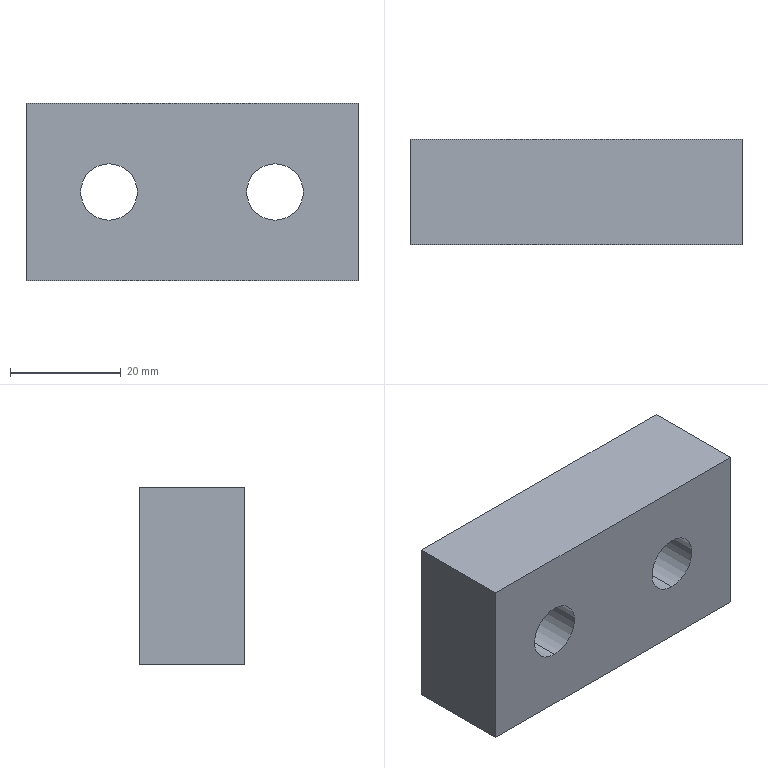Part | SolidWorks | features FlatPattern 1, HoleWzd 1, SMBaseFlange 1, SheetMetal 1 | 1 solid | 10 faces | box 60 x 19 x 32 mm | volume 33375 mm3 | plane 6 | cylinder 4 | commonest cylinder face diameters 10.2 x4
STEP:
#1=CARTESIAN_POINT('',(-15.,-19.,-5.1));
#2=VERTEX_POINT('',#1);
#3=CARTESIAN_POINT('',(-15.,-19.,5.1));
#4=VERTEX_POINT('',#3);
#5=CARTESIAN_POINT('',(-15.,-19.,0.));
#6=DIRECTION('',(0.,1.,0.));
#7=DIRECTION('',(0.,0.,1.));
#8=AXIS2_PLACEMENT_3D('',#5,#6,#7);
#9=CIRCLE('',#8,5.1);
#10=EDGE_CURVE('',#2,#4,#9,.T.);
#11=ORIENTED_EDGE('',*,*,#10,.F.);
#12=CARTESIAN_POINT('',(-15.,0.,-5.1));
#13=VERTEX_POINT('',#12);
#14=CARTESIAN_POINT('',(-15.,0.,-5.1));
#15=DIRECTION('',(0.,1.,0.));
#16=VECTOR('',#15,1000.);
#17=LINE('',#14,#16);
#18=EDGE_CURVE('',#2,#13,#17,.T.);
#19=ORIENTED_EDGE('',*,*,#18,.T.);
#20=CARTESIAN_POINT('',(-15.,0.,5.1));
#21=VERTEX_POINT('',#20);
#22=CARTESIAN_POINT('',(-15.,0.,0.));
#23=DIRECTION('',(0.,1.,0.));
#24=DIRECTION('',(0.,0.,1.));
#25=AXIS2_PLACEMENT_3D('',#22,#23,#24);
#26=CIRCLE('',#25,5.1);
#27=EDGE_CURVE('',#13,#21,#26,.T.);
#28=ORIENTED_EDGE('',*,*,#27,.T.);
#29=CARTESIAN_POINT('',(-15.,0.,5.1));
#30=DIRECTION('',(0.,1.,0.));
#31=VECTOR('',#30,1000.);
#32=LINE('',#29,#31);
#33=EDGE_CURVE('',#4,#21,#32,.T.);
#34=ORIENTED_EDGE('',*,*,#33,.F.);
#35=EDGE_LOOP('',(#11,#19,#28,#34));
#36=FACE_OUTER_BOUND('',#35,.T.);
#37=CARTESIAN_POINT('',(-15.,0.,0.));
#38=DIRECTION('',(0.,1.,0.));
#39=DIRECTION('',(0.,0.,1.));
#40=AXIS2_PLACEMENT_3D('',#37,#38,#39);
#41=CYLINDRICAL_SURFACE('',#40,5.1);
#42=ADVANCED_FACE('',(#36),#41,.F.);
#43=CARTESIAN_POINT('',(15.,-19.,-5.1));
#44=VERTEX_POINT('',#43);
#45=CARTESIAN_POINT('',(15.,-19.,5.1));
#46=VERTEX_POINT('',#45);
#47=CARTESIAN_POINT('',(15.,-19.,0.));
#48=DIRECTION('',(0.,1.,0.));
#49=DIRECTION('',(0.,0.,1.));
#50=AXIS2_PLACEMENT_3D('',#47,#48,#49);
#51=CIRCLE('',#50,5.1);
#52=EDGE_CURVE('',#44,#46,#51,.T.);
#53=ORIENTED_EDGE('',*,*,#52,.F.);
#54=CARTESIAN_POINT('',(15.,0.,-5.1));
#55=VERTEX_POINT('',#54);
#56=CARTESIAN_POINT('',(15.,0.,-5.1));
#57=DIRECTION('',(0.,1.,0.));
#58=VECTOR('',#57,1000.);
#59=LINE('',#56,#58);
#60=EDGE_CURVE('',#44,#55,#59,.T.);
#61=ORIENTED_EDGE('',*,*,#60,.T.);
#62=CARTESIAN_POINT('',(15.,0.,5.1));
#63=VERTEX_POINT('',#62);
#64=CARTESIAN_POINT('',(15.,0.,0.));
#65=DIRECTION('',(0.,1.,0.));
#66=DIRECTION('',(0.,0.,1.));
#67=AXIS2_PLACEMENT_3D('',#64,#65,#66);
#68=CIRCLE('',#67,5.1);
#69=EDGE_CURVE('',#55,#63,#68,.T.);
#70=ORIENTED_EDGE('',*,*,#69,.T.);
#71=CARTESIAN_POINT('',(15.,0.,5.1));
#72=DIRECTION('',(0.,1.,0.));
#73=VECTOR('',#72,1000.);
#74=LINE('',#71,#73);
#75=EDGE_CURVE('',#46,#63,#74,.T.);
#76=ORIENTED_EDGE('',*,*,#75,.F.);
#77=EDGE_LOOP('',(#53,#61,#70,#76));
#78=FACE_OUTER_BOUND('',#77,.T.);
#79=CARTESIAN_POINT('',(15.,0.,0.));
#80=DIRECTION('',(0.,1.,0.));
#81=DIRECTION('',(0.,0.,1.));
#82=AXIS2_PLACEMENT_3D('',#79,#80,#81);
#83=CYLINDRICAL_SURFACE('',#82,5.1);
#84=ADVANCED_FACE('',(#78),#83,.F.);
#85=CARTESIAN_POINT('',(30.,0.,16.));
#86=VERTEX_POINT('',#85);
#87=CARTESIAN_POINT('',(30.,0.,-16.));
#88=VERTEX_POINT('',#87);
#89=CARTESIAN_POINT('',(30.,0.,-16.));
#90=DIRECTION('',(0.,0.,-1.));
#91=VECTOR('',#90,1000.);
#92=LINE('',#89,#91);
#93=EDGE_CURVE('',#86,#88,#92,.T.);
#94=ORIENTED_EDGE('',*,*,#93,.F.);
#95=CARTESIAN_POINT('',(30.,-19.,16.));
#96=VERTEX_POINT('',#95);
#97=CARTESIAN_POINT('',(30.,-19.,16.));
#98=DIRECTION('',(0.,1.,0.));
#99=VECTOR('',#98,1000.);
#100=LINE('',#97,#99);
#101=EDGE_CURVE('',#96,#86,#100,.T.);
#102=ORIENTED_EDGE('',*,*,#101,.F.);
#103=CARTESIAN_POINT('',(30.,-19.,-16.));
#104=VERTEX_POINT('',#103);
#105=CARTESIAN_POINT('',(30.,-19.,-16.));
#106=DIRECTION('',(0.,0.,-1.));
#107=VECTOR('',#106,1000.);
#108=LINE('',#105,#107);
#109=EDGE_CURVE('',#96,#104,#108,.T.);
#110=ORIENTED_EDGE('',*,*,#109,.T.);
#111=CARTESIAN_POINT('',(30.,-19.,-16.));
#112=DIRECTION('',(0.,1.,0.));
#113=VECTOR('',#112,1000.);
#114=LINE('',#111,#113);
#115=EDGE_CURVE('',#104,#88,#114,.T.);
#116=ORIENTED_EDGE('',*,*,#115,.T.);
#117=EDGE_LOOP('',(#94,#102,#110,#116));
#118=FACE_OUTER_BOUND('',#117,.T.);
#119=CARTESIAN_POINT('',(30.,-19.,-16.));
#120=DIRECTION('',(1.,0.,0.));
#121=DIRECTION('',(0.,0.,-1.));
#122=AXIS2_PLACEMENT_3D('',#119,#120,#121);
#123=PLANE('',#122);
#124=ADVANCED_FACE('',(#118),#123,.T.);
#125=CARTESIAN_POINT('',(-30.,0.,16.));
#126=VERTEX_POINT('',#125);
#127=CARTESIAN_POINT('',(-30.,0.,16.));
#128=DIRECTION('',(1.,0.,0.));
#129=VECTOR('',#128,1000.);
#130=LINE('',#127,#129);
#131=EDGE_CURVE('',#126,#86,#130,.T.);
#132=ORIENTED_EDGE('',*,*,#131,.F.);
#133=CARTESIAN_POINT('',(-30.,-19.,16.));
#134=VERTEX_POINT('',#133);
#135=CARTESIAN_POINT('',(-30.,-19.,16.));
#136=DIRECTION('',(0.,1.,0.));
#137=VECTOR('',#136,1000.);
#138=LINE('',#135,#137);
#139=EDGE_CURVE('',#134,#126,#138,.T.);
#140=ORIENTED_EDGE('',*,*,#139,.F.);
#141=CARTESIAN_POINT('',(-30.,-19.,16.));
#142=DIRECTION('',(1.,0.,0.));
#143=VECTOR('',#142,1000.);
#144=LINE('',#141,#143);
#145=EDGE_CURVE('',#134,#96,#144,.T.);
#146=ORIENTED_EDGE('',*,*,#145,.T.);
#147=ORIENTED_EDGE('',*,*,#101,.T.);
#148=EDGE_LOOP('',(#132,#140,#146,#147));
#149=FACE_OUTER_BOUND('',#148,.T.);
#150=CARTESIAN_POINT('',(-30.,-19.,16.));
#151=DIRECTION('',(0.,0.,1.));
#152=DIRECTION('',(1.,0.,0.));
#153=AXIS2_PLACEMENT_3D('',#150,#151,#152);
#154=PLANE('',#153);
#155=ADVANCED_FACE('',(#149),#154,.T.);
#156=CARTESIAN_POINT('',(-30.,0.,-16.));
#157=VERTEX_POINT('',#156);
#158=CARTESIAN_POINT('',(-30.,0.,-16.));
#159=DIRECTION('',(0.,0.,1.));
#160=VECTOR('',#159,1000.);
#161=LINE('',#158,#160);
#162=EDGE_CURVE('',#157,#126,#161,.T.);
#163=ORIENTED_EDGE('',*,*,#162,.F.);
#164=CARTESIAN_POINT('',(-30.,-19.,-16.));
#165=VERTEX_POINT('',#164);
#166=CARTESIAN_POINT('',(-30.,-19.,-16.));
#167=DIRECTION('',(0.,1.,0.));
#168=VECTOR('',#167,1000.);
#169=LINE('',#166,#168);
#170=EDGE_CURVE('',#165,#157,#169,.T.);
#171=ORIENTED_EDGE('',*,*,#170,.F.);
#172=CARTESIAN_POINT('',(-30.,-19.,-16.));
#173=DIRECTION('',(0.,0.,1.));
#174=VECTOR('',#173,1000.);
#175=LINE('',#172,#174);
#176=EDGE_CURVE('',#165,#134,#175,.T.);
#177=ORIENTED_EDGE('',*,*,#176,.T.);
#178=ORIENTED_EDGE('',*,*,#139,.T.);
#179=EDGE_LOOP('',(#163,#171,#177,#178));
#180=FACE_OUTER_BOUND('',#179,.T.);
#181=CARTESIAN_POINT('',(-30.,-19.,-16.));
#182=DIRECTION('',(-1.,0.,0.));
#183=DIRECTION('',(0.,0.,1.));
#184=AXIS2_PLACEMENT_3D('',#181,#182,#183);
#185=PLANE('',#184);
#186=ADVANCED_FACE('',(#180),#185,.T.);
#187=CARTESIAN_POINT('',(-30.,0.,-16.));
#188=DIRECTION('',(-1.,0.,0.));
#189=VECTOR('',#188,1000.);
#190=LINE('',#187,#189);
#191=EDGE_CURVE('',#88,#157,#190,.T.);
#192=ORIENTED_EDGE('',*,*,#191,.F.);
#193=ORIENTED_EDGE('',*,*,#115,.F.);
#194=CARTESIAN_POINT('',(-30.,-19.,-16.));
#195=DIRECTION('',(-1.,0.,0.));
#196=VECTOR('',#195,1000.);
#197=LINE('',#194,#196);
#198=EDGE_CURVE('',#104,#165,#197,.T.);
#199=ORIENTED_EDGE('',*,*,#198,.T.);
#200=ORIENTED_EDGE('',*,*,#170,.T.);
#201=EDGE_LOOP('',(#192,#193,#199,#200));
#202=FACE_OUTER_BOUND('',#201,.T.);
#203=CARTESIAN_POINT('',(-30.,-19.,-16.));
#204=DIRECTION('',(0.,0.,-1.));
#205=DIRECTION('',(-1.,0.,0.));
#206=AXIS2_PLACEMENT_3D('',#203,#204,#205);
#207=PLANE('',#206);
#208=ADVANCED_FACE('',(#202),#207,.T.);
#209=CARTESIAN_POINT('',(-15.,-19.,0.));
#210=DIRECTION('',(0.,1.,0.));
#211=DIRECTION('',(0.,0.,1.));
#212=AXIS2_PLACEMENT_3D('',#209,#210,#211);
#213=CIRCLE('',#212,5.1);
#214=EDGE_CURVE('',#4,#2,#213,.T.);
#215=ORIENTED_EDGE('',*,*,#214,.T.);
#216=ORIENTED_EDGE('',*,*,#10,.T.);
#217=EDGE_LOOP('',(#215,#216));
#218=FACE_BOUND('',#217,.T.);
#219=CARTESIAN_POINT('',(15.,-19.,0.));
#220=DIRECTION('',(0.,1.,0.));
#221=DIRECTION('',(0.,0.,1.));
#222=AXIS2_PLACEMENT_3D('',#219,#220,#221);
#223=CIRCLE('',#222,5.1);
#224=EDGE_CURVE('',#46,#44,#223,.T.);
#225=ORIENTED_EDGE('',*,*,#224,.T.);
#226=ORIENTED_EDGE('',*,*,#52,.T.);
#227=EDGE_LOOP('',(#225,#226));
#228=FACE_BOUND('',#227,.T.);
#229=ORIENTED_EDGE('',*,*,#109,.F.);
#230=ORIENTED_EDGE('',*,*,#145,.F.);
#231=ORIENTED_EDGE('',*,*,#176,.F.);
#232=ORIENTED_EDGE('',*,*,#198,.F.);
#233=EDGE_LOOP('',(#229,#230,#231,#232));
#234=FACE_OUTER_BOUND('',#233,.T.);
#235=CARTESIAN_POINT('',(0.,-19.,0.));
#236=DIRECTION('',(0.,1.,0.));
#237=DIRECTION('',(0.,0.,1.));
#238=AXIS2_PLACEMENT_3D('',#235,#236,#237);
#239=PLANE('',#238);
#240=ADVANCED_FACE('',(#218,#228,#234),#239,.F.);
#241=CARTESIAN_POINT('',(-15.,0.,0.));
#242=DIRECTION('',(0.,1.,0.));
#243=DIRECTION('',(0.,0.,1.));
#244=AXIS2_PLACEMENT_3D('',#241,#242,#243);
#245=CIRCLE('',#244,5.1);
#246=EDGE_CURVE('',#21,#13,#245,.T.);
#247=ORIENTED_EDGE('',*,*,#246,.F.);
#248=ORIENTED_EDGE('',*,*,#27,.F.);
#249=EDGE_LOOP('',(#247,#248));
#250=FACE_BOUND('',#249,.T.);
#251=CARTESIAN_POINT('',(15.,0.,0.));
#252=DIRECTION('',(0.,1.,0.));
#253=DIRECTION('',(0.,0.,1.));
#254=AXIS2_PLACEMENT_3D('',#251,#252,#253);
#255=CIRCLE('',#254,5.1);
#256=EDGE_CURVE('',#63,#55,#255,.T.);
#257=ORIENTED_EDGE('',*,*,#256,.F.);
#258=ORIENTED_EDGE('',*,*,#69,.F.);
#259=EDGE_LOOP('',(#257,#258));
#260=FACE_BOUND('',#259,.T.);
#261=ORIENTED_EDGE('',*,*,#93,.T.);
#262=ORIENTED_EDGE('',*,*,#191,.T.);
#263=ORIENTED_EDGE('',*,*,#162,.T.);
#264=ORIENTED_EDGE('',*,*,#131,.T.);
#265=EDGE_LOOP('',(#261,#262,#263,#264));
#266=FACE_OUTER_BOUND('',#265,.T.);
#267=CARTESIAN_POINT('',(0.,0.,0.));
#268=DIRECTION('',(0.,1.,0.));
#269=DIRECTION('',(0.,0.,1.));
#270=AXIS2_PLACEMENT_3D('',#267,#268,#269);
#271=PLANE('',#270);
#272=ADVANCED_FACE('',(#250,#260,#266),#271,.T.);
#273=ORIENTED_EDGE('',*,*,#60,.F.);
#274=ORIENTED_EDGE('',*,*,#224,.F.);
#275=ORIENTED_EDGE('',*,*,#75,.T.);
#276=ORIENTED_EDGE('',*,*,#256,.T.);
#277=EDGE_LOOP('',(#273,#274,#275,#276));
#278=FACE_OUTER_BOUND('',#277,.T.);
#279=CARTESIAN_POINT('',(15.,0.,0.));
#280=DIRECTION('',(0.,1.,0.));
#281=DIRECTION('',(0.,0.,1.));
#282=AXIS2_PLACEMENT_3D('',#279,#280,#281);
#283=CYLINDRICAL_SURFACE('',#282,5.1);
#284=ADVANCED_FACE('',(#278),#283,.F.);
#285=ORIENTED_EDGE('',*,*,#18,.F.);
#286=ORIENTED_EDGE('',*,*,#214,.F.);
#287=ORIENTED_EDGE('',*,*,#33,.T.);
#288=ORIENTED_EDGE('',*,*,#246,.T.);
#289=EDGE_LOOP('',(#285,#286,#287,#288));
#290=FACE_OUTER_BOUND('',#289,.T.);
#291=CARTESIAN_POINT('',(-15.,0.,0.));
#292=DIRECTION('',(0.,1.,0.));
#293=DIRECTION('',(0.,0.,1.));
#294=AXIS2_PLACEMENT_3D('',#291,#292,#293);
#295=CYLINDRICAL_SURFACE('',#294,5.1);
#296=ADVANCED_FACE('',(#290),#295,.F.);
#297=CLOSED_SHELL('',(#42,#84,#124,#155,#186,#208,#240,#272,#284,#296));
#298=MANIFOLD_SOLID_BREP('',#297);
#299=CARTESIAN_POINT('',(0.,0.,0.));
#300=DIRECTION('',(0.,0.,1.));
#301=DIRECTION('',(1.,0.,0.));
#302=AXIS2_PLACEMENT_3D('',#299,#300,#301);
#303=(LENGTH_UNIT()NAMED_UNIT(*)SI_UNIT(.MILLI.,.METRE.));
#304=UNCERTAINTY_MEASURE_WITH_UNIT(LENGTH_MEASURE(0.00001),#303,'','');
#305=(NAMED_UNIT(*)PLANE_ANGLE_UNIT()SI_UNIT($,.RADIAN.));
#306=(NAMED_UNIT(*)SI_UNIT($,.STERADIAN.)SOLID_ANGLE_UNIT());
#307=(GEOMETRIC_REPRESENTATION_CONTEXT(3)GLOBAL_UNCERTAINTY_ASSIGNED_CONTEXT((#304))GLOBAL_UNIT_ASSIGNED_CONTEXT((#303,#305,#306))REPRESENTATION_CONTEXT('',''));
#308=ADVANCED_BREP_SHAPE_REPRESENTATION('',(#298,#302),#307);